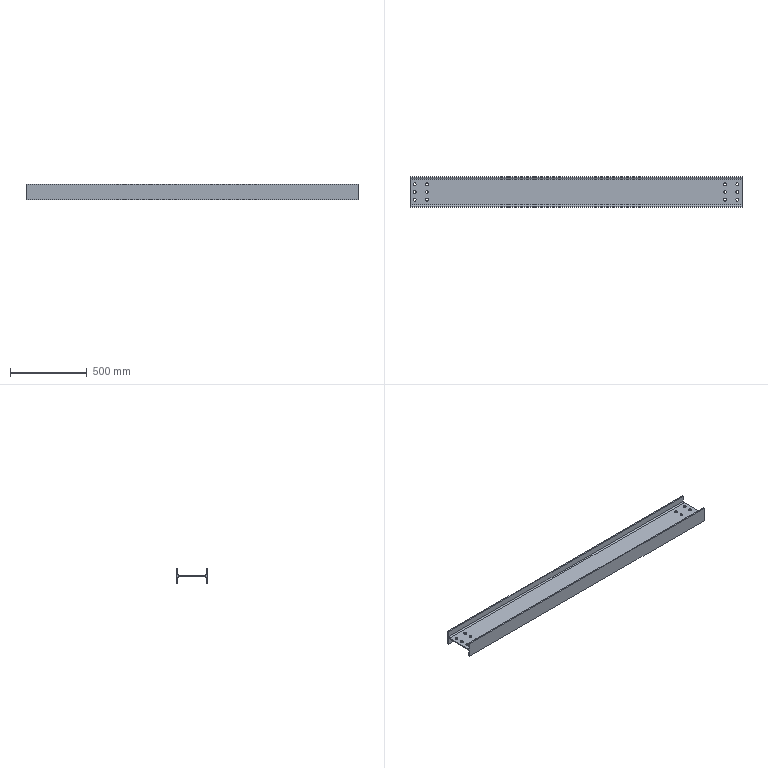Part | STEP file | 计量主梁7主体_Default<As Machined> | 1 solid | 42 faces | box 2170 x 200 x 100 mm | volume 5768543 mm3 | cylinder 28 | plane 14 | commonest cylinder face diameters 19 x24 16 x4